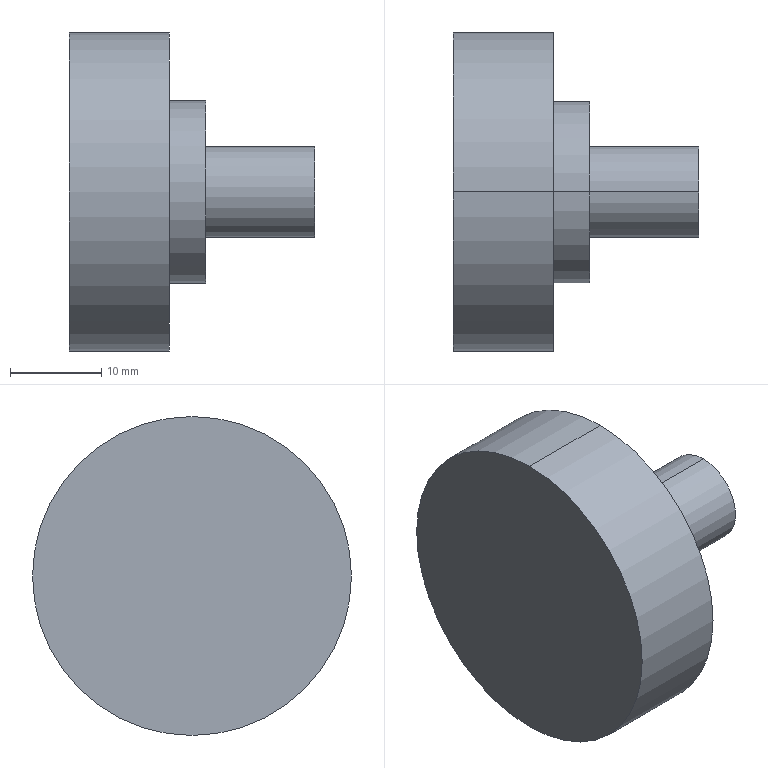Part | NX | features BREP 1 | 1 solid | 10 faces | box 27 x 35 x 35 mm | volume 12782 mm3 | cylinder 6 | plane 4 | commonest cylinder face diameters 10 x2 20 x2 35 x2
STEP:
#1=CARTESIAN_POINT('',(27.,0.,5.));
#2=VERTEX_POINT('',#1);
#3=CARTESIAN_POINT('',(27.,0.,-5.));
#4=VERTEX_POINT('',#3);
#5=CARTESIAN_POINT('',(27.,0.,0.));
#6=DIRECTION('',(-1.,0.,0.));
#7=DIRECTION('',(0.,0.,1.));
#8=AXIS2_PLACEMENT_3D('',#5,#6,#7);
#9=CIRCLE('',#8,5.);
#10=EDGE_CURVE('',#2,#4,#9,.T.);
#11=ORIENTED_EDGE('',*,*,#10,.T.);
#12=CARTESIAN_POINT('',(15.,0.,-5.));
#13=VERTEX_POINT('',#12);
#14=CARTESIAN_POINT('',(0.,0.,-5.));
#15=DIRECTION('',(-1.,0.,0.));
#16=VECTOR('',#15,1000.);
#17=LINE('',#14,#16);
#18=EDGE_CURVE('',#13,#4,#17,.F.);
#19=ORIENTED_EDGE('',*,*,#18,.F.);
#20=CARTESIAN_POINT('',(15.,0.,5.));
#21=VERTEX_POINT('',#20);
#22=CARTESIAN_POINT('',(15.,0.,0.));
#23=DIRECTION('',(-1.,0.,0.));
#24=DIRECTION('',(0.,0.,1.));
#25=AXIS2_PLACEMENT_3D('',#22,#23,#24);
#26=CIRCLE('',#25,5.);
#27=EDGE_CURVE('',#21,#13,#26,.T.);
#28=ORIENTED_EDGE('',*,*,#27,.F.);
#29=CARTESIAN_POINT('',(0.,0.,5.));
#30=DIRECTION('',(-1.,0.,0.));
#31=VECTOR('',#30,1000.);
#32=LINE('',#29,#31);
#33=EDGE_CURVE('',#21,#2,#32,.F.);
#34=ORIENTED_EDGE('',*,*,#33,.T.);
#35=EDGE_LOOP('',(#11,#19,#28,#34));
#36=FACE_BOUND('',#35,.T.);
#37=CARTESIAN_POINT('',(0.,0.,0.));
#38=DIRECTION('',(-1.,0.,0.));
#39=DIRECTION('',(0.,0.,1.));
#40=AXIS2_PLACEMENT_3D('',#37,#38,#39);
#41=CYLINDRICAL_SURFACE('',#40,5.);
#42=ADVANCED_FACE('',(#36),#41,.T.);
#43=CARTESIAN_POINT('',(15.,0.,10.));
#44=VERTEX_POINT('',#43);
#45=CARTESIAN_POINT('',(15.,0.,-10.));
#46=VERTEX_POINT('',#45);
#47=CARTESIAN_POINT('',(15.,0.,0.));
#48=DIRECTION('',(-1.,0.,0.));
#49=DIRECTION('',(0.,0.,1.));
#50=AXIS2_PLACEMENT_3D('',#47,#48,#49);
#51=CIRCLE('',#50,10.);
#52=EDGE_CURVE('',#44,#46,#51,.T.);
#53=ORIENTED_EDGE('',*,*,#52,.T.);
#54=CARTESIAN_POINT('',(11.,0.,-10.));
#55=VERTEX_POINT('',#54);
#56=CARTESIAN_POINT('',(0.,0.,-10.));
#57=DIRECTION('',(-1.,0.,0.));
#58=VECTOR('',#57,1000.);
#59=LINE('',#56,#58);
#60=EDGE_CURVE('',#55,#46,#59,.F.);
#61=ORIENTED_EDGE('',*,*,#60,.F.);
#62=CARTESIAN_POINT('',(11.,0.,10.));
#63=VERTEX_POINT('',#62);
#64=CARTESIAN_POINT('',(11.,0.,0.));
#65=DIRECTION('',(-1.,0.,0.));
#66=DIRECTION('',(0.,0.,1.));
#67=AXIS2_PLACEMENT_3D('',#64,#65,#66);
#68=CIRCLE('',#67,10.);
#69=EDGE_CURVE('',#63,#55,#68,.T.);
#70=ORIENTED_EDGE('',*,*,#69,.F.);
#71=CARTESIAN_POINT('',(0.,0.,10.));
#72=DIRECTION('',(-1.,0.,0.));
#73=VECTOR('',#72,1000.);
#74=LINE('',#71,#73);
#75=EDGE_CURVE('',#63,#44,#74,.F.);
#76=ORIENTED_EDGE('',*,*,#75,.T.);
#77=EDGE_LOOP('',(#53,#61,#70,#76));
#78=FACE_BOUND('',#77,.T.);
#79=CARTESIAN_POINT('',(0.,0.,0.));
#80=DIRECTION('',(-1.,0.,0.));
#81=DIRECTION('',(0.,0.,1.));
#82=AXIS2_PLACEMENT_3D('',#79,#80,#81);
#83=CYLINDRICAL_SURFACE('',#82,10.);
#84=ADVANCED_FACE('',(#78),#83,.T.);
#85=CARTESIAN_POINT('',(11.,0.,17.5));
#86=VERTEX_POINT('',#85);
#87=CARTESIAN_POINT('',(11.,0.,-17.5));
#88=VERTEX_POINT('',#87);
#89=CARTESIAN_POINT('',(11.,0.,0.));
#90=DIRECTION('',(-1.,0.,0.));
#91=DIRECTION('',(0.,0.,1.));
#92=AXIS2_PLACEMENT_3D('',#89,#90,#91);
#93=CIRCLE('',#92,17.5);
#94=EDGE_CURVE('',#86,#88,#93,.T.);
#95=ORIENTED_EDGE('',*,*,#94,.T.);
#96=CARTESIAN_POINT('',(0.,0.,-17.5));
#97=VERTEX_POINT('',#96);
#98=CARTESIAN_POINT('',(0.,0.,-17.5));
#99=DIRECTION('',(-1.,0.,0.));
#100=VECTOR('',#99,1000.);
#101=LINE('',#98,#100);
#102=EDGE_CURVE('',#97,#88,#101,.F.);
#103=ORIENTED_EDGE('',*,*,#102,.F.);
#104=CARTESIAN_POINT('',(0.,0.,17.5));
#105=VERTEX_POINT('',#104);
#106=CARTESIAN_POINT('',(0.,0.,0.));
#107=DIRECTION('',(-1.,0.,0.));
#108=DIRECTION('',(0.,0.,1.));
#109=AXIS2_PLACEMENT_3D('',#106,#107,#108);
#110=CIRCLE('',#109,17.5);
#111=EDGE_CURVE('',#105,#97,#110,.T.);
#112=ORIENTED_EDGE('',*,*,#111,.F.);
#113=CARTESIAN_POINT('',(0.,0.,17.5));
#114=DIRECTION('',(-1.,0.,0.));
#115=VECTOR('',#114,1000.);
#116=LINE('',#113,#115);
#117=EDGE_CURVE('',#105,#86,#116,.F.);
#118=ORIENTED_EDGE('',*,*,#117,.T.);
#119=EDGE_LOOP('',(#95,#103,#112,#118));
#120=FACE_BOUND('',#119,.T.);
#121=CARTESIAN_POINT('',(0.,0.,0.));
#122=DIRECTION('',(-1.,0.,0.));
#123=DIRECTION('',(0.,0.,1.));
#124=AXIS2_PLACEMENT_3D('',#121,#122,#123);
#125=CYLINDRICAL_SURFACE('',#124,17.5);
#126=ADVANCED_FACE('',(#120),#125,.T.);
#127=ORIENTED_EDGE('',*,*,#111,.T.);
#128=CARTESIAN_POINT('',(0.,0.,0.));
#129=DIRECTION('',(-1.,0.,0.));
#130=DIRECTION('',(0.,0.,1.));
#131=AXIS2_PLACEMENT_3D('',#128,#129,#130);
#132=CIRCLE('',#131,17.5);
#133=EDGE_CURVE('',#97,#105,#132,.T.);
#134=ORIENTED_EDGE('',*,*,#133,.T.);
#135=EDGE_LOOP('',(#127,#134));
#136=FACE_BOUND('',#135,.T.);
#137=CARTESIAN_POINT('',(0.,0.,0.));
#138=DIRECTION('',(1.,0.,0.));
#139=DIRECTION('',(0.,1.,0.));
#140=AXIS2_PLACEMENT_3D('',#137,#138,#139);
#141=PLANE('',#140);
#142=ADVANCED_FACE('',(#136),#141,.F.);
#143=ORIENTED_EDGE('',*,*,#102,.T.);
#144=CARTESIAN_POINT('',(11.,0.,0.));
#145=DIRECTION('',(-1.,0.,0.));
#146=DIRECTION('',(0.,0.,1.));
#147=AXIS2_PLACEMENT_3D('',#144,#145,#146);
#148=CIRCLE('',#147,17.5);
#149=EDGE_CURVE('',#88,#86,#148,.T.);
#150=ORIENTED_EDGE('',*,*,#149,.T.);
#151=ORIENTED_EDGE('',*,*,#117,.F.);
#152=ORIENTED_EDGE('',*,*,#133,.F.);
#153=EDGE_LOOP('',(#143,#150,#151,#152));
#154=FACE_BOUND('',#153,.T.);
#155=CARTESIAN_POINT('',(0.,0.,0.));
#156=DIRECTION('',(-1.,0.,0.));
#157=DIRECTION('',(0.,0.,1.));
#158=AXIS2_PLACEMENT_3D('',#155,#156,#157);
#159=CYLINDRICAL_SURFACE('',#158,17.5);
#160=ADVANCED_FACE('',(#154),#159,.T.);
#161=ORIENTED_EDGE('',*,*,#94,.F.);
#162=ORIENTED_EDGE('',*,*,#149,.F.);
#163=EDGE_LOOP('',(#161,#162));
#164=FACE_BOUND('',#163,.T.);
#165=ORIENTED_EDGE('',*,*,#69,.T.);
#166=CARTESIAN_POINT('',(11.,0.,0.));
#167=DIRECTION('',(-1.,0.,0.));
#168=DIRECTION('',(0.,0.,1.));
#169=AXIS2_PLACEMENT_3D('',#166,#167,#168);
#170=CIRCLE('',#169,10.);
#171=EDGE_CURVE('',#55,#63,#170,.T.);
#172=ORIENTED_EDGE('',*,*,#171,.T.);
#173=EDGE_LOOP('',(#165,#172));
#174=FACE_BOUND('',#173,.T.);
#175=CARTESIAN_POINT('',(11.,17.5,0.));
#176=DIRECTION('',(-1.,0.,0.));
#177=DIRECTION('',(0.,0.,1.));
#178=AXIS2_PLACEMENT_3D('',#175,#176,#177);
#179=PLANE('',#178);
#180=ADVANCED_FACE('',(#164,#174),#179,.F.);
#181=ORIENTED_EDGE('',*,*,#60,.T.);
#182=CARTESIAN_POINT('',(15.,0.,0.));
#183=DIRECTION('',(-1.,0.,0.));
#184=DIRECTION('',(0.,0.,1.));
#185=AXIS2_PLACEMENT_3D('',#182,#183,#184);
#186=CIRCLE('',#185,10.);
#187=EDGE_CURVE('',#46,#44,#186,.T.);
#188=ORIENTED_EDGE('',*,*,#187,.T.);
#189=ORIENTED_EDGE('',*,*,#75,.F.);
#190=ORIENTED_EDGE('',*,*,#171,.F.);
#191=EDGE_LOOP('',(#181,#188,#189,#190));
#192=FACE_BOUND('',#191,.T.);
#193=CARTESIAN_POINT('',(0.,0.,0.));
#194=DIRECTION('',(-1.,0.,0.));
#195=DIRECTION('',(0.,0.,1.));
#196=AXIS2_PLACEMENT_3D('',#193,#194,#195);
#197=CYLINDRICAL_SURFACE('',#196,10.);
#198=ADVANCED_FACE('',(#192),#197,.T.);
#199=ORIENTED_EDGE('',*,*,#52,.F.);
#200=ORIENTED_EDGE('',*,*,#187,.F.);
#201=EDGE_LOOP('',(#199,#200));
#202=FACE_BOUND('',#201,.T.);
#203=ORIENTED_EDGE('',*,*,#27,.T.);
#204=CARTESIAN_POINT('',(15.,0.,0.));
#205=DIRECTION('',(-1.,0.,0.));
#206=DIRECTION('',(0.,0.,1.));
#207=AXIS2_PLACEMENT_3D('',#204,#205,#206);
#208=CIRCLE('',#207,5.);
#209=EDGE_CURVE('',#13,#21,#208,.T.);
#210=ORIENTED_EDGE('',*,*,#209,.T.);
#211=EDGE_LOOP('',(#203,#210));
#212=FACE_BOUND('',#211,.T.);
#213=CARTESIAN_POINT('',(15.,10.,0.));
#214=DIRECTION('',(-1.,0.,0.));
#215=DIRECTION('',(0.,0.,1.));
#216=AXIS2_PLACEMENT_3D('',#213,#214,#215);
#217=PLANE('',#216);
#218=ADVANCED_FACE('',(#202,#212),#217,.F.);
#219=ORIENTED_EDGE('',*,*,#18,.T.);
#220=CARTESIAN_POINT('',(27.,0.,0.));
#221=DIRECTION('',(-1.,0.,0.));
#222=DIRECTION('',(0.,0.,1.));
#223=AXIS2_PLACEMENT_3D('',#220,#221,#222);
#224=CIRCLE('',#223,5.);
#225=EDGE_CURVE('',#4,#2,#224,.T.);
#226=ORIENTED_EDGE('',*,*,#225,.T.);
#227=ORIENTED_EDGE('',*,*,#33,.F.);
#228=ORIENTED_EDGE('',*,*,#209,.F.);
#229=EDGE_LOOP('',(#219,#226,#227,#228));
#230=FACE_BOUND('',#229,.T.);
#231=CARTESIAN_POINT('',(0.,0.,0.));
#232=DIRECTION('',(-1.,0.,0.));
#233=DIRECTION('',(0.,0.,1.));
#234=AXIS2_PLACEMENT_3D('',#231,#232,#233);
#235=CYLINDRICAL_SURFACE('',#234,5.);
#236=ADVANCED_FACE('',(#230),#235,.T.);
#237=ORIENTED_EDGE('',*,*,#10,.F.);
#238=ORIENTED_EDGE('',*,*,#225,.F.);
#239=EDGE_LOOP('',(#237,#238));
#240=FACE_BOUND('',#239,.T.);
#241=CARTESIAN_POINT('',(27.,5.,0.));
#242=DIRECTION('',(-1.,0.,0.));
#243=DIRECTION('',(0.,0.,1.));
#244=AXIS2_PLACEMENT_3D('',#241,#242,#243);
#245=PLANE('',#244);
#246=ADVANCED_FACE('',(#240),#245,.F.);
#247=CLOSED_SHELL('',(#42,#84,#126,#142,#160,#180,#198,#218,#236,#246));
#248=MANIFOLD_SOLID_BREP('',#247);
#249=(LENGTH_UNIT()NAMED_UNIT(*)SI_UNIT(.MILLI.,.METRE.));
#250=UNCERTAINTY_MEASURE_WITH_UNIT(LENGTH_MEASURE(0.00001),#249,'','');
#251=(NAMED_UNIT(*)PLANE_ANGLE_UNIT()SI_UNIT($,.RADIAN.));
#252=(NAMED_UNIT(*)SI_UNIT($,.STERADIAN.)SOLID_ANGLE_UNIT());
#253=(GEOMETRIC_REPRESENTATION_CONTEXT(3)GLOBAL_UNCERTAINTY_ASSIGNED_CONTEXT((#250))GLOBAL_UNIT_ASSIGNED_CONTEXT((#249,#251,#252))REPRESENTATION_CONTEXT('',''));
#254=ADVANCED_BREP_SHAPE_REPRESENTATION('',(#248),#253);